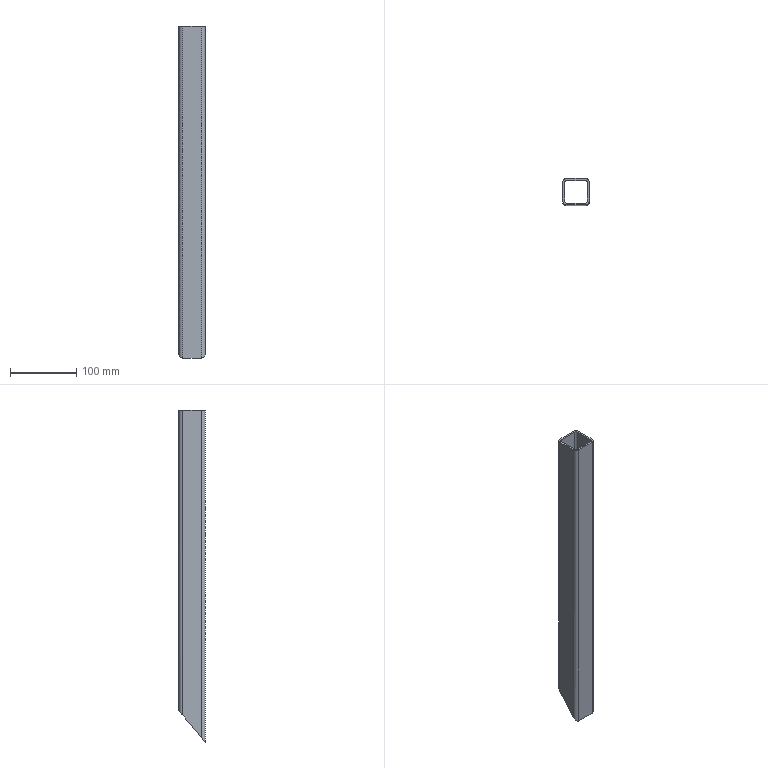Part | STEP file | DIN 59 410 - 40x40x2.9-300 | 1 solid | 18 faces | box 40 x 40 x 500 mm | volume 194610 mm3 | plane 10 | cylinder 8 | commonest cylinder face diameters 5.8 x4 11.6 x4